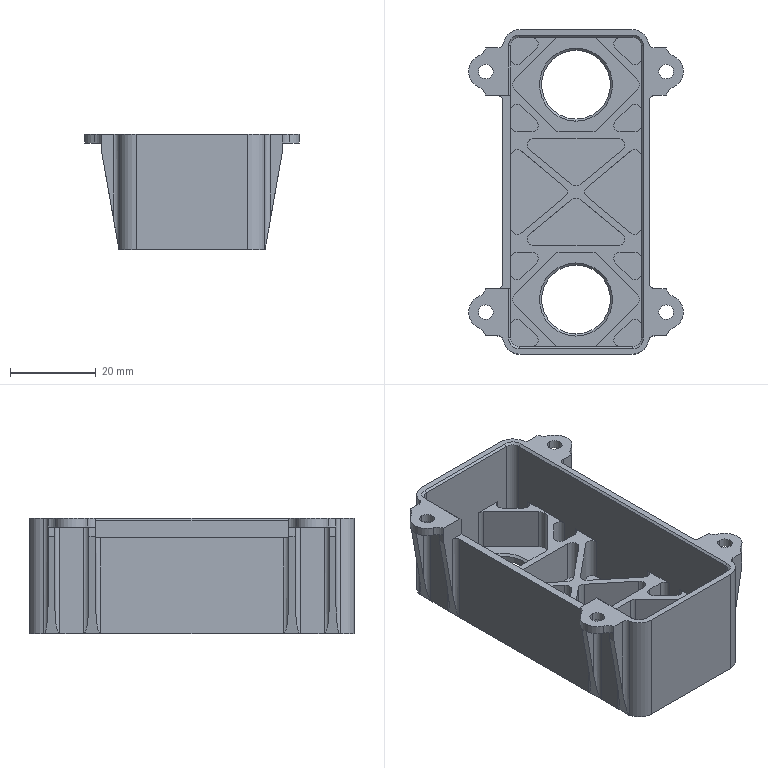NC program | NX | posted with a generic post | part box 50 x 75.58 x 26.8 mm
Lines 6055 to 6157 of 37241:
(ZLEVEL_PROFILE_COPY_1_COPY_COPY_1_COPY_COPY_1_COPY , TOOL : D10JING)
N12090 T14 M6
N12092 G54
N12094 G17 G0 G90 X-27.71 Y0.704 S9500 M3
N12096 G43 Z30. H14
N12098 Z-1.
N12100 G94 G1 Z-2. F1000.
N12102 G3 X-28. Y0. R1.
N12104 G1 Y-0.009 F1200.
N12106 G3 X-24.991 Y-3. R3.
N12108 X-28. Y0. R-3.
N12110 X-27.71 Y-0.704 R1.
N12112 G1 Z-1.
N12114 G0 Z30.
N12116 X27.71
N12118 Z-1.
N12120 G1 Z-2. F1000.
N12122 G3 X28. Y0. R1.
N12124 X25. Y3. R3. F1200.
N12126 X28. Y0. R-3.
N12128 X27.71 Y0.704 R1.
N12130 G1 Z-1.
N12132 G0 Z30.
(ZLEVEL_PROFILE_COPY_1_COPY_COPY_1_COPY_COPY_1 , TOOL : D10JING)
N12134 X42.972 Y13.575
N12136 Z-12.4
N12138 G1 Z-13.4 F1000.
N12140 G3 X42.79 Y13. R1.
N12142 G1 Y-13. F1200.
N12144 G2 X38.285 Y-20.797 R9.
N12146 X33.5 Y-24.363 R4.997
N12148 G1 X32.
N12150 G2 X28. Y-22.363 R5.014
N12152 X24. Y-24.363 R5.01
N12154 G1 X22.495
N12156 G2 X18.758 Y-22.67 R4.972
N12158 X18.219 Y-22. R10.027
N12160 G1 X-18.219
N12162 G2 X-19.543 Y-23.389 R5.914
N12164 X-22.448 Y-24.363 R4.822
N12166 G1 X-24.
N12168 G2 X-28. Y-22.363 R5.009
N12170 X-32. Y-24.363 R5.015
N12172 G1 X-33.5
N12174 G2 X-38.285 Y-20.797 R4.996
N12176 X-42.79 Y-13. R9.
N12178 G1 Y13.
N12180 G2 X-38.285 Y20.797 R9.
N12182 X-33.5 Y24.363 R4.996
N12184 G1 X-32.
N12186 G2 X-28. Y22.363 R5.014
N12188 X-24. Y24.363 R5.01
N12190 G1 X-22.495
N12192 G2 X-18.758 Y22.67 R4.972
N12194 X-18.219 Y22. R10.027
N12196 G1 X18.219
N12198 G2 X19.543 Y23.389 R5.914
N12200 X22.448 Y24.363 R4.822
N12202 G1 X24.
N12204 G2 X28. Y22.363 R5.009
N12206 X32. Y24.363 R5.015
N12208 G1 X33.5
N12210 G2 X38.285 Y20.797 R4.997
N12212 X42.79 Y13. R9.
N12214 G3 X42.99 Y12.4 R1.
N12216 G1 Z-12.4
N12218 G0 Z30.
N12220 X42.972 Y13.575
N12222 Z-25.8
N12224 G1 Z-26.8 F1000.
N12226 G3 X42.79 Y13. R1.
N12228 G1 Y-13. F1200.
N12230 G2 X38.5 Y-20.669 R9.
N12232 G1 Y-21.
N12234 G2 X35.841 Y-25.418 R5.
N12236 X20.159 Y-25.418 R9.
N12238 X17.601 Y-22. R5.
N12240 G1 X-17.601
N12242 G2 X-20.159 Y-25.418 R5.
N12244 X-35.841 Y-25.418 R9.
N12246 X-38.5 Y-21. R5.
N12248 G1 Y-20.669
N12250 G2 X-42.79 Y-13. R9.
N12252 G1 Y13.
N12254 G2 X-38.5 Y20.669 R9.
N12256 G1 Y21.
N12258 G2 X-35.841 Y25.418 R5.
N12260 X-20.159 Y25.418 R9.
N12262 X-17.601 Y22. R5.
N12264 G1 X17.601
N12266 G2 X20.159 Y25.418 R5.
N12268 X35.841 Y25.418 R9.
N12270 X38.5 Y21. R5.
N12272 G1 Y20.669
N12274 G2 X42.79 Y13. R9.
N12276 G3 X42.99 Y12.4 R1.
N12278 G1 Z-25.8
N12280 G0 Z30.
N12282 M5